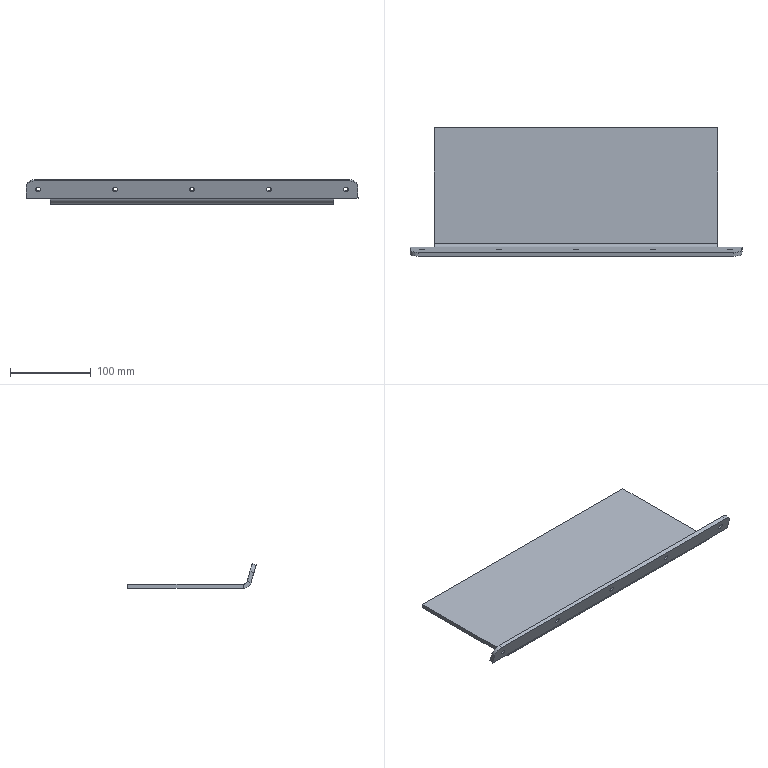Part | SolidWorks | features 3DProfileFeature 1, EdgeFlange 1, Fillet 1, FlatPattern 1, HoleWzd 1, LPattern 1, SMBaseFlange 1, SheetMetal 1 | 1 solid | 38 faces | box 410 x 158.498 x 30.188 mm | volume 311527 mm3 | cylinder 14 | plane 14 | cone 10 | commonest cylinder face diameters 6 x10 20 x3 10 x1
STEP:
#1=CARTESIAN_POINT('',(190.,-81.218,21.139));
#2=VERTEX_POINT('',#1);
#3=CARTESIAN_POINT('',(190.,-79.518,15.385));
#4=VERTEX_POINT('',#3);
#5=CARTESIAN_POINT('',(190.,-80.368,18.262));
#6=DIRECTION('',(0.,-0.959,-0.2833));
#7=DIRECTION('',(0.,0.2833,-0.959));
#8=AXIS2_PLACEMENT_3D('',#5,#6,#7);
#9=CIRCLE('',#8,3.);
#10=EDGE_CURVE('',#2,#4,#9,.T.);
#11=ORIENTED_EDGE('',*,*,#10,.F.);
#12=CARTESIAN_POINT('',(190.,-81.249,21.156));
#13=VERTEX_POINT('',#12);
#14=CARTESIAN_POINT('',(190.,-81.249,21.156));
#15=DIRECTION('',(0.,-0.8784,0.4778));
#16=VECTOR('',#15,1000.);
#17=LINE('',#14,#16);
#18=EDGE_CURVE('',#2,#13,#17,.T.);
#19=ORIENTED_EDGE('',*,*,#18,.T.);
#20=CARTESIAN_POINT('',(190.,-79.535,15.354));
#21=VERTEX_POINT('',#20);
#22=CARTESIAN_POINT('',(190.,-80.392,18.255));
#23=DIRECTION('',(0.,-0.959,-0.2833));
#24=DIRECTION('',(0.,0.2833,-0.959));
#25=AXIS2_PLACEMENT_3D('',#22,#23,#24);
#26=CIRCLE('',#25,3.025);
#27=EDGE_CURVE('',#13,#21,#26,.T.);
#28=ORIENTED_EDGE('',*,*,#27,.T.);
#29=CARTESIAN_POINT('',(190.,-79.535,15.354));
#30=DIRECTION('',(0.,-0.4778,-0.8784));
#31=VECTOR('',#30,1000.);
#32=LINE('',#29,#31);
#33=EDGE_CURVE('',#4,#21,#32,.T.);
#34=ORIENTED_EDGE('',*,*,#33,.F.);
#35=EDGE_LOOP('',(#11,#19,#28,#34));
#36=FACE_OUTER_BOUND('',#35,.T.);
#37=CARTESIAN_POINT('',(190.,-80.392,18.255));
#38=DIRECTION('',(0.,-0.959,-0.2833));
#39=DIRECTION('',(0.,0.2833,-0.959));
#40=AXIS2_PLACEMENT_3D('',#37,#38,#39);
#41=CONICAL_SURFACE('',#40,3.025,0.7854);
#42=ADVANCED_FACE('',(#36),#41,.F.);
#43=CARTESIAN_POINT('',(190.,-76.447,22.549));
#44=VERTEX_POINT('',#43);
#45=CARTESIAN_POINT('',(190.,-74.747,16.794));
#46=VERTEX_POINT('',#45);
#47=CARTESIAN_POINT('',(190.,-75.597,19.671));
#48=DIRECTION('',(0.,-0.959,-0.2833));
#49=DIRECTION('',(0.,0.2833,-0.959));
#50=AXIS2_PLACEMENT_3D('',#47,#48,#49);
#51=CIRCLE('',#50,3.);
#52=EDGE_CURVE('',#44,#46,#51,.T.);
#53=ORIENTED_EDGE('',*,*,#52,.F.);
#54=CARTESIAN_POINT('',(190.,-81.242,21.132));
#55=DIRECTION('',(0.,-0.959,-0.2833));
#56=VECTOR('',#55,1000.);
#57=LINE('',#54,#56);
#58=EDGE_CURVE('',#44,#2,#57,.T.);
#59=ORIENTED_EDGE('',*,*,#58,.T.);
#60=ORIENTED_EDGE('',*,*,#10,.T.);
#61=CARTESIAN_POINT('',(190.,-79.542,15.378));
#62=DIRECTION('',(0.,-0.959,-0.2833));
#63=VECTOR('',#62,1000.);
#64=LINE('',#61,#63);
#65=EDGE_CURVE('',#46,#4,#64,.T.);
#66=ORIENTED_EDGE('',*,*,#65,.F.);
#67=EDGE_LOOP('',(#53,#59,#60,#66));
#68=FACE_OUTER_BOUND('',#67,.T.);
#69=CARTESIAN_POINT('',(190.,-80.392,18.255));
#70=DIRECTION('',(0.,-0.959,-0.2833));
#71=DIRECTION('',(0.,0.2833,-0.959));
#72=AXIS2_PLACEMENT_3D('',#69,#70,#71);
#73=CYLINDRICAL_SURFACE('',#72,3.);
#74=ADVANCED_FACE('',(#68),#73,.F.);
#75=CARTESIAN_POINT('',(95.,-81.218,21.139));
#76=VERTEX_POINT('',#75);
#77=CARTESIAN_POINT('',(95.,-79.518,15.385));
#78=VERTEX_POINT('',#77);
#79=CARTESIAN_POINT('',(95.,-80.368,18.262));
#80=DIRECTION('',(0.,-0.959,-0.2833));
#81=DIRECTION('',(0.,0.2833,-0.959));
#82=AXIS2_PLACEMENT_3D('',#79,#80,#81);
#83=CIRCLE('',#82,3.);
#84=EDGE_CURVE('',#76,#78,#83,.T.);
#85=ORIENTED_EDGE('',*,*,#84,.F.);
#86=CARTESIAN_POINT('',(95.,-81.249,21.156));
#87=VERTEX_POINT('',#86);
#88=CARTESIAN_POINT('',(95.,-81.249,21.156));
#89=DIRECTION('',(0.,-0.8784,0.4778));
#90=VECTOR('',#89,1000.);
#91=LINE('',#88,#90);
#92=EDGE_CURVE('',#76,#87,#91,.T.);
#93=ORIENTED_EDGE('',*,*,#92,.T.);
#94=CARTESIAN_POINT('',(95.,-79.535,15.354));
#95=VERTEX_POINT('',#94);
#96=CARTESIAN_POINT('',(95.,-80.392,18.255));
#97=DIRECTION('',(0.,-0.959,-0.2833));
#98=DIRECTION('',(0.,0.2833,-0.959));
#99=AXIS2_PLACEMENT_3D('',#96,#97,#98);
#100=CIRCLE('',#99,3.025);
#101=EDGE_CURVE('',#87,#95,#100,.T.);
#102=ORIENTED_EDGE('',*,*,#101,.T.);
#103=CARTESIAN_POINT('',(95.,-79.535,15.354));
#104=DIRECTION('',(0.,-0.4778,-0.8784));
#105=VECTOR('',#104,1000.);
#106=LINE('',#103,#105);
#107=EDGE_CURVE('',#78,#95,#106,.T.);
#108=ORIENTED_EDGE('',*,*,#107,.F.);
#109=EDGE_LOOP('',(#85,#93,#102,#108));
#110=FACE_OUTER_BOUND('',#109,.T.);
#111=CARTESIAN_POINT('',(95.,-80.392,18.255));
#112=DIRECTION('',(0.,-0.959,-0.2833));
#113=DIRECTION('',(0.,0.2833,-0.959));
#114=AXIS2_PLACEMENT_3D('',#111,#112,#113);
#115=CONICAL_SURFACE('',#114,3.025,0.7854);
#116=ADVANCED_FACE('',(#110),#115,.F.);
#117=CARTESIAN_POINT('',(95.,-76.447,22.549));
#118=VERTEX_POINT('',#117);
#119=CARTESIAN_POINT('',(95.,-74.747,16.794));
#120=VERTEX_POINT('',#119);
#121=CARTESIAN_POINT('',(95.,-75.597,19.671));
#122=DIRECTION('',(0.,-0.959,-0.2833));
#123=DIRECTION('',(0.,0.2833,-0.959));
#124=AXIS2_PLACEMENT_3D('',#121,#122,#123);
#125=CIRCLE('',#124,3.);
#126=EDGE_CURVE('',#118,#120,#125,.T.);
#127=ORIENTED_EDGE('',*,*,#126,.F.);
#128=CARTESIAN_POINT('',(95.,-81.242,21.132));
#129=DIRECTION('',(0.,-0.959,-0.2833));
#130=VECTOR('',#129,1000.);
#131=LINE('',#128,#130);
#132=EDGE_CURVE('',#118,#76,#131,.T.);
#133=ORIENTED_EDGE('',*,*,#132,.T.);
#134=ORIENTED_EDGE('',*,*,#84,.T.);
#135=CARTESIAN_POINT('',(95.,-79.542,15.378));
#136=DIRECTION('',(0.,-0.959,-0.2833));
#137=VECTOR('',#136,1000.);
#138=LINE('',#135,#137);
#139=EDGE_CURVE('',#120,#78,#138,.T.);
#140=ORIENTED_EDGE('',*,*,#139,.F.);
#141=EDGE_LOOP('',(#127,#133,#134,#140));
#142=FACE_OUTER_BOUND('',#141,.T.);
#143=CARTESIAN_POINT('',(95.,-80.392,18.255));
#144=DIRECTION('',(0.,-0.959,-0.2833));
#145=DIRECTION('',(0.,0.2833,-0.959));
#146=AXIS2_PLACEMENT_3D('',#143,#144,#145);
#147=CYLINDRICAL_SURFACE('',#146,3.);
#148=ADVANCED_FACE('',(#142),#147,.F.);
#149=CARTESIAN_POINT('',(0.,-81.218,21.139));
#150=VERTEX_POINT('',#149);
#151=CARTESIAN_POINT('',(0.,-79.518,15.385));
#152=VERTEX_POINT('',#151);
#153=CARTESIAN_POINT('',(0.,-80.368,18.262));
#154=DIRECTION('',(0.,-0.959,-0.2833));
#155=DIRECTION('',(0.,0.2833,-0.959));
#156=AXIS2_PLACEMENT_3D('',#153,#154,#155);
#157=CIRCLE('',#156,3.);
#158=EDGE_CURVE('',#150,#152,#157,.T.);
#159=ORIENTED_EDGE('',*,*,#158,.F.);
#160=CARTESIAN_POINT('',(0.,-81.249,21.156));
#161=VERTEX_POINT('',#160);
#162=CARTESIAN_POINT('',(0.,-81.249,21.156));
#163=DIRECTION('',(0.,-0.8784,0.4778));
#164=VECTOR('',#163,1000.);
#165=LINE('',#162,#164);
#166=EDGE_CURVE('',#150,#161,#165,.T.);
#167=ORIENTED_EDGE('',*,*,#166,.T.);
#168=CARTESIAN_POINT('',(0.,-79.535,15.354));
#169=VERTEX_POINT('',#168);
#170=CARTESIAN_POINT('',(0.,-80.392,18.255));
#171=DIRECTION('',(0.,-0.959,-0.2833));
#172=DIRECTION('',(0.,0.2833,-0.959));
#173=AXIS2_PLACEMENT_3D('',#170,#171,#172);
#174=CIRCLE('',#173,3.025);
#175=EDGE_CURVE('',#161,#169,#174,.T.);
#176=ORIENTED_EDGE('',*,*,#175,.T.);
#177=CARTESIAN_POINT('',(0.,-79.535,15.354));
#178=DIRECTION('',(0.,-0.4778,-0.8784));
#179=VECTOR('',#178,1000.);
#180=LINE('',#177,#179);
#181=EDGE_CURVE('',#152,#169,#180,.T.);
#182=ORIENTED_EDGE('',*,*,#181,.F.);
#183=EDGE_LOOP('',(#159,#167,#176,#182));
#184=FACE_OUTER_BOUND('',#183,.T.);
#185=CARTESIAN_POINT('',(0.,-80.392,18.255));
#186=DIRECTION('',(0.,-0.959,-0.2833));
#187=DIRECTION('',(0.,0.2833,-0.959));
#188=AXIS2_PLACEMENT_3D('',#185,#186,#187);
#189=CONICAL_SURFACE('',#188,3.025,0.7854);
#190=ADVANCED_FACE('',(#184),#189,.F.);
#191=CARTESIAN_POINT('',(0.,-76.447,22.549));
#192=VERTEX_POINT('',#191);
#193=CARTESIAN_POINT('',(0.,-74.747,16.794));
#194=VERTEX_POINT('',#193);
#195=CARTESIAN_POINT('',(0.,-75.597,19.671));
#196=DIRECTION('',(0.,-0.959,-0.2833));
#197=DIRECTION('',(0.,0.2833,-0.959));
#198=AXIS2_PLACEMENT_3D('',#195,#196,#197);
#199=CIRCLE('',#198,3.);
#200=EDGE_CURVE('',#192,#194,#199,.T.);
#201=ORIENTED_EDGE('',*,*,#200,.F.);
#202=CARTESIAN_POINT('',(0.,-81.242,21.132));
#203=DIRECTION('',(0.,-0.959,-0.2833));
#204=VECTOR('',#203,1000.);
#205=LINE('',#202,#204);
#206=EDGE_CURVE('',#192,#150,#205,.T.);
#207=ORIENTED_EDGE('',*,*,#206,.T.);
#208=ORIENTED_EDGE('',*,*,#158,.T.);
#209=CARTESIAN_POINT('',(0.,-79.542,15.378));
#210=DIRECTION('',(0.,-0.959,-0.2833));
#211=VECTOR('',#210,1000.);
#212=LINE('',#209,#211);
#213=EDGE_CURVE('',#194,#152,#212,.T.);
#214=ORIENTED_EDGE('',*,*,#213,.F.);
#215=EDGE_LOOP('',(#201,#207,#208,#214));
#216=FACE_OUTER_BOUND('',#215,.T.);
#217=CARTESIAN_POINT('',(0.,-80.392,18.255));
#218=DIRECTION('',(0.,-0.959,-0.2833));
#219=DIRECTION('',(0.,0.2833,-0.959));
#220=AXIS2_PLACEMENT_3D('',#217,#218,#219);
#221=CYLINDRICAL_SURFACE('',#220,3.);
#222=ADVANCED_FACE('',(#216),#221,.F.);
#223=CARTESIAN_POINT('',(-95.,-81.218,21.139));
#224=VERTEX_POINT('',#223);
#225=CARTESIAN_POINT('',(-95.,-79.518,15.385));
#226=VERTEX_POINT('',#225);
#227=CARTESIAN_POINT('',(-95.,-80.368,18.262));
#228=DIRECTION('',(0.,-0.959,-0.2833));
#229=DIRECTION('',(0.,0.2833,-0.959));
#230=AXIS2_PLACEMENT_3D('',#227,#228,#229);
#231=CIRCLE('',#230,3.);
#232=EDGE_CURVE('',#224,#226,#231,.T.);
#233=ORIENTED_EDGE('',*,*,#232,.F.);
#234=CARTESIAN_POINT('',(-95.,-81.249,21.156));
#235=VERTEX_POINT('',#234);
#236=CARTESIAN_POINT('',(-95.,-81.249,21.156));
#237=DIRECTION('',(0.,-0.8784,0.4778));
#238=VECTOR('',#237,1000.);
#239=LINE('',#236,#238);
#240=EDGE_CURVE('',#224,#235,#239,.T.);
#241=ORIENTED_EDGE('',*,*,#240,.T.);
#242=CARTESIAN_POINT('',(-95.,-79.535,15.354));
#243=VERTEX_POINT('',#242);
#244=CARTESIAN_POINT('',(-95.,-80.392,18.255));
#245=DIRECTION('',(0.,-0.959,-0.2833));
#246=DIRECTION('',(0.,0.2833,-0.959));
#247=AXIS2_PLACEMENT_3D('',#244,#245,#246);
#248=CIRCLE('',#247,3.025);
#249=EDGE_CURVE('',#235,#243,#248,.T.);
#250=ORIENTED_EDGE('',*,*,#249,.T.);
#251=CARTESIAN_POINT('',(-95.,-79.535,15.354));
#252=DIRECTION('',(0.,-0.4778,-0.8784));
#253=VECTOR('',#252,1000.);
#254=LINE('',#251,#253);
#255=EDGE_CURVE('',#226,#243,#254,.T.);
#256=ORIENTED_EDGE('',*,*,#255,.F.);
#257=EDGE_LOOP('',(#233,#241,#250,#256));
#258=FACE_OUTER_BOUND('',#257,.T.);
#259=CARTESIAN_POINT('',(-95.,-80.392,18.255));
#260=DIRECTION('',(0.,-0.959,-0.2833));
#261=DIRECTION('',(0.,0.2833,-0.959));
#262=AXIS2_PLACEMENT_3D('',#259,#260,#261);
#263=CONICAL_SURFACE('',#262,3.025,0.7854);
#264=ADVANCED_FACE('',(#258),#263,.F.);
#265=CARTESIAN_POINT('',(-95.,-76.447,22.549));
#266=VERTEX_POINT('',#265);
#267=CARTESIAN_POINT('',(-95.,-74.747,16.794));
#268=VERTEX_POINT('',#267);
#269=CARTESIAN_POINT('',(-95.,-75.597,19.671));
#270=DIRECTION('',(0.,-0.959,-0.2833));
#271=DIRECTION('',(0.,0.2833,-0.959));
#272=AXIS2_PLACEMENT_3D('',#269,#270,#271);
#273=CIRCLE('',#272,3.);
#274=EDGE_CURVE('',#266,#268,#273,.T.);
#275=ORIENTED_EDGE('',*,*,#274,.F.);
#276=CARTESIAN_POINT('',(-95.,-81.242,21.132));
#277=DIRECTION('',(0.,-0.959,-0.2833));
#278=VECTOR('',#277,1000.);
#279=LINE('',#276,#278);
#280=EDGE_CURVE('',#266,#224,#279,.T.);
#281=ORIENTED_EDGE('',*,*,#280,.T.);
#282=ORIENTED_EDGE('',*,*,#232,.T.);
#283=CARTESIAN_POINT('',(-95.,-79.542,15.378));
#284=DIRECTION('',(0.,-0.959,-0.2833));
#285=VECTOR('',#284,1000.);
#286=LINE('',#283,#285);
#287=EDGE_CURVE('',#268,#226,#286,.T.);
#288=ORIENTED_EDGE('',*,*,#287,.F.);
#289=EDGE_LOOP('',(#275,#281,#282,#288));
#290=FACE_OUTER_BOUND('',#289,.T.);
#291=CARTESIAN_POINT('',(-95.,-80.392,18.255));
#292=DIRECTION('',(0.,-0.959,-0.2833));
#293=DIRECTION('',(0.,0.2833,-0.959));
#294=AXIS2_PLACEMENT_3D('',#291,#292,#293);
#295=CYLINDRICAL_SURFACE('',#294,3.);
#296=ADVANCED_FACE('',(#290),#295,.F.);
#297=CARTESIAN_POINT('',(-190.,-81.218,21.139));
#298=VERTEX_POINT('',#297);
#299=CARTESIAN_POINT('',(-190.,-79.518,15.385));
#300=VERTEX_POINT('',#299);
#301=CARTESIAN_POINT('',(-190.,-80.368,18.262));
#302=DIRECTION('',(0.,-0.959,-0.2833));
#303=DIRECTION('',(0.,0.2833,-0.959));
#304=AXIS2_PLACEMENT_3D('',#301,#302,#303);
#305=CIRCLE('',#304,3.);
#306=EDGE_CURVE('',#298,#300,#305,.T.);
#307=ORIENTED_EDGE('',*,*,#306,.F.);
#308=CARTESIAN_POINT('',(-190.,-81.249,21.156));
#309=VERTEX_POINT('',#308);
#310=CARTESIAN_POINT('',(-190.,-81.249,21.156));
#311=DIRECTION('',(0.,-0.8784,0.4778));
#312=VECTOR('',#311,1000.);
#313=LINE('',#310,#312);
#314=EDGE_CURVE('',#298,#309,#313,.T.);
#315=ORIENTED_EDGE('',*,*,#314,.T.);
#316=CARTESIAN_POINT('',(-190.,-79.535,15.354));
#317=VERTEX_POINT('',#316);
#318=CARTESIAN_POINT('',(-190.,-80.392,18.255));
#319=DIRECTION('',(0.,-0.959,-0.2833));
#320=DIRECTION('',(0.,0.2833,-0.959));
#321=AXIS2_PLACEMENT_3D('',#318,#319,#320);
#322=CIRCLE('',#321,3.025);
#323=EDGE_CURVE('',#309,#317,#322,.T.);
#324=ORIENTED_EDGE('',*,*,#323,.T.);
#325=CARTESIAN_POINT('',(-190.,-79.535,15.354));
#326=DIRECTION('',(0.,-0.4778,-0.8784));
#327=VECTOR('',#326,1000.);
#328=LINE('',#325,#327);
#329=EDGE_CURVE('',#300,#317,#328,.T.);
#330=ORIENTED_EDGE('',*,*,#329,.F.);
#331=EDGE_LOOP('',(#307,#315,#324,#330));
#332=FACE_OUTER_BOUND('',#331,.T.);
#333=CARTESIAN_POINT('',(-190.,-80.392,18.255));
#334=DIRECTION('',(0.,-0.959,-0.2833));
#335=DIRECTION('',(0.,0.2833,-0.959));
#336=AXIS2_PLACEMENT_3D('',#333,#334,#335);
#337=CONICAL_SURFACE('',#336,3.025,0.7854);
#338=ADVANCED_FACE('',(#332),#337,.F.);
#339=CARTESIAN_POINT('',(-190.,-76.447,22.549));
#340=VERTEX_POINT('',#339);
#341=CARTESIAN_POINT('',(-190.,-74.747,16.794));
#342=VERTEX_POINT('',#341);
#343=CARTESIAN_POINT('',(-190.,-75.597,19.671));
#344=DIRECTION('',(0.,-0.959,-0.2833));
#345=DIRECTION('',(0.,0.2833,-0.959));
#346=AXIS2_PLACEMENT_3D('',#343,#344,#345);
#347=CIRCLE('',#346,3.);
#348=EDGE_CURVE('',#340,#342,#347,.T.);
#349=ORIENTED_EDGE('',*,*,#348,.F.);
#350=CARTESIAN_POINT('',(-190.,-81.242,21.132));
#351=DIRECTION('',(0.,-0.959,-0.2833));
#352=VECTOR('',#351,1000.);
#353=LINE('',#350,#352);
#354=EDGE_CURVE('',#340,#298,#353,.T.);
#355=ORIENTED_EDGE('',*,*,#354,.T.);
#356=ORIENTED_EDGE('',*,*,#306,.T.);
#357=CARTESIAN_POINT('',(-190.,-79.542,15.378));
#358=DIRECTION('',(0.,-0.959,-0.2833));
#359=VECTOR('',#358,1000.);
#360=LINE('',#357,#359);
#361=EDGE_CURVE('',#342,#300,#360,.T.);
#362=ORIENTED_EDGE('',*,*,#361,.F.);
#363=EDGE_LOOP('',(#349,#355,#356,#362));
#364=FACE_OUTER_BOUND('',#363,.T.);
#365=CARTESIAN_POINT('',(-190.,-80.392,18.255));
#366=DIRECTION('',(0.,-0.959,-0.2833));
#367=DIRECTION('',(0.,0.2833,-0.959));
#368=AXIS2_PLACEMENT_3D('',#365,#366,#367);
#369=CYLINDRICAL_SURFACE('',#368,3.);
#370=ADVANCED_FACE('',(#364),#369,.F.);
#371=CARTESIAN_POINT('',(175.,-67.527,5.));
#372=VERTEX_POINT('',#371);
#373=CARTESIAN_POINT('',(175.,-67.527,0.));
#374=VERTEX_POINT('',#373);
#375=CARTESIAN_POINT('',(175.,-67.527,5.));
#376=DIRECTION('',(0.,0.,-1.));
#377=VECTOR('',#376,1000.);
#378=LINE('',#375,#377);
#379=EDGE_CURVE('',#372,#374,#378,.T.);
#380=ORIENTED_EDGE('',*,*,#379,.T.);
#381=CARTESIAN_POINT('',(175.,75.,0.));
#382=VERTEX_POINT('',#381);
#383=CARTESIAN_POINT('',(175.,75.,0.));
#384=DIRECTION('',(0.,1.,0.));
#385=VECTOR('',#384,1000.);
#386=LINE('',#383,#385);
#387=EDGE_CURVE('',#374,#382,#386,.T.);
#388=ORIENTED_EDGE('',*,*,#387,.T.);
#389=CARTESIAN_POINT('',(175.,75.,5.));
#390=VERTEX_POINT('',#389);
#391=CARTESIAN_POINT('',(175.,75.,5.));
#392=DIRECTION('',(0.,0.,-1.));
#393=VECTOR('',#392,1000.);
#394=LINE('',#391,#393);
#395=EDGE_CURVE('',#390,#382,#394,.T.);
#396=ORIENTED_EDGE('',*,*,#395,.F.);
#397=CARTESIAN_POINT('',(175.,75.,5.));
#398=DIRECTION('',(0.,1.,0.));
#399=VECTOR('',#398,1000.);
#400=LINE('',#397,#399);
#401=EDGE_CURVE('',#372,#390,#400,.T.);
#402=ORIENTED_EDGE('',*,*,#401,.F.);
#403=EDGE_LOOP('',(#380,#388,#396,#402));
#404=FACE_OUTER_BOUND('',#403,.T.);
#405=CARTESIAN_POINT('',(175.,75.,5.));
#406=DIRECTION('',(-1.,0.,0.));
#407=DIRECTION('',(0.,0.,1.));
#408=AXIS2_PLACEMENT_3D('',#405,#406,#407);
#409=PLANE('',#408);
#410=ADVANCED_FACE('',(#404),#409,.F.);
#411=CARTESIAN_POINT('',(-175.,-67.527,5.));
#412=VERTEX_POINT('',#411);
#413=CARTESIAN_POINT('',(-175.,-67.527,0.));
#414=VERTEX_POINT('',#413);
#415=CARTESIAN_POINT('',(-175.,-67.527,5.));
#416=DIRECTION('',(0.,0.,-1.));
#417=VECTOR('',#416,1000.);
#418=LINE('',#415,#417);
#419=EDGE_CURVE('',#412,#414,#418,.T.);
#420=ORIENTED_EDGE('',*,*,#419,.F.);
#421=CARTESIAN_POINT('',(-175.,75.,5.));
#422=VERTEX_POINT('',#421);
#423=CARTESIAN_POINT('',(-175.,75.,5.));
#424=DIRECTION('',(0.,-1.,0.));
#425=VECTOR('',#424,1000.);
#426=LINE('',#423,#425);
#427=EDGE_CURVE('',#422,#412,#426,.T.);
#428=ORIENTED_EDGE('',*,*,#427,.F.);
#429=CARTESIAN_POINT('',(-175.,75.,0.));
#430=VERTEX_POINT('',#429);
#431=CARTESIAN_POINT('',(-175.,75.,5.));
#432=DIRECTION('',(0.,0.,-1.));
#433=VECTOR('',#432,1000.);
#434=LINE('',#431,#433);
#435=EDGE_CURVE('',#422,#430,#434,.T.);
#436=ORIENTED_EDGE('',*,*,#435,.T.);
#437=CARTESIAN_POINT('',(-175.,75.,0.));
#438=DIRECTION('',(0.,-1.,0.));
#439=VECTOR('',#438,1000.);
#440=LINE('',#437,#439);
#441=EDGE_CURVE('',#430,#414,#440,.T.);
#442=ORIENTED_EDGE('',*,*,#441,.T.);
#443=EDGE_LOOP('',(#420,#428,#436,#442));
#444=FACE_OUTER_BOUND('',#443,.T.);
#445=CARTESIAN_POINT('',(-175.,75.,5.));
#446=DIRECTION('',(1.,0.,0.));
#447=DIRECTION('',(0.,0.,-1.));
#448=AXIS2_PLACEMENT_3D('',#445,#446,#447);
#449=PLANE('',#448);
#450=ADVANCED_FACE('',(#444),#449,.F.);
#451=ORIENTED_EDGE('',*,*,#427,.T.);
#452=CARTESIAN_POINT('',(175.,-67.527,5.));
#453=DIRECTION('',(-1.,0.,0.));
#454=VECTOR('',#453,1000.);
#455=LINE('',#452,#454);
#456=EDGE_CURVE('',#372,#412,#455,.T.);
#457=ORIENTED_EDGE('',*,*,#456,.F.);
#458=ORIENTED_EDGE('',*,*,#401,.T.);
#459=CARTESIAN_POINT('',(-175.,75.,5.));
#460=DIRECTION('',(-1.,0.,0.));
#461=VECTOR('',#460,1000.);
#462=LINE('',#459,#461);
#463=EDGE_CURVE('',#390,#422,#462,.T.);
#464=ORIENTED_EDGE('',*,*,#463,.T.);
#465=EDGE_LOOP('',(#451,#457,#458,#464));
#466=FACE_OUTER_BOUND('',#465,.T.);
#467=CARTESIAN_POINT('',(0.,0.,5.));
#468=DIRECTION('',(0.,0.,1.));
#469=DIRECTION('',(1.,0.,0.));
#470=AXIS2_PLACEMENT_3D('',#467,#468,#469);
#471=PLANE('',#470);
#472=ADVANCED_FACE('',(#466),#471,.T.);
#473=CARTESIAN_POINT('',(175.,-67.527,0.));
#474=DIRECTION('',(-1.,0.,0.));
#475=VECTOR('',#474,1000.);
#476=LINE('',#473,#475);
#477=EDGE_CURVE('',#374,#414,#476,.T.);
#478=ORIENTED_EDGE('',*,*,#477,.T.);
#479=ORIENTED_EDGE('',*,*,#441,.F.);
#480=CARTESIAN_POINT('',(-175.,75.,0.));
#481=DIRECTION('',(-1.,0.,0.));
#482=VECTOR('',#481,1000.);
#483=LINE('',#480,#482);
#484=EDGE_CURVE('',#382,#430,#483,.T.);
#485=ORIENTED_EDGE('',*,*,#484,.F.);
#486=ORIENTED_EDGE('',*,*,#387,.F.);
#487=EDGE_LOOP('',(#478,#479,#485,#486));
#488=FACE_OUTER_BOUND('',#487,.T.);
#489=CARTESIAN_POINT('',(0.,0.,0.));
#490=DIRECTION('',(0.,0.,1.));
#491=DIRECTION('',(1.,0.,0.));
#492=AXIS2_PLACEMENT_3D('',#489,#490,#491);
#493=PLANE('',#492);
#494=ADVANCED_FACE('',(#488),#493,.F.);
#495=ORIENTED_EDGE('',*,*,#484,.T.);
#496=ORIENTED_EDGE('',*,*,#435,.F.);
#497=ORIENTED_EDGE('',*,*,#463,.F.);
#498=ORIENTED_EDGE('',*,*,#395,.T.);
#499=EDGE_LOOP('',(#495,#496,#497,#498));
#500=FACE_OUTER_BOUND('',#499,.T.);
#501=CARTESIAN_POINT('',(-175.,75.,5.));
#502=DIRECTION('',(0.,-1.,0.));
#503=DIRECTION('',(0.,0.,-1.));
#504=AXIS2_PLACEMENT_3D('',#501,#502,#503);
#505=PLANE('',#504);
#506=ADVANCED_FACE('',(#500),#505,.F.);
#507=CARTESIAN_POINT('',(-175.,-72.322,8.584));
#508=VERTEX_POINT('',#507);
#509=CARTESIAN_POINT('',(-175.,-77.117,7.167));
#510=VERTEX_POINT('',#509);
#511=CARTESIAN_POINT('',(-175.,-72.322,8.584));
#512=DIRECTION('',(0.,-0.959,-0.2833));
#513=VECTOR('',#512,1000.);
#514=LINE('',#511,#513);
#515=EDGE_CURVE('',#508,#510,#514,.T.);
#516=ORIENTED_EDGE('',*,*,#515,.F.);
#517=CARTESIAN_POINT('',(-175.,-67.527,10.));
#518=DIRECTION('',(-1.,0.,0.));
#519=DIRECTION('',(0.,0.,-1.));
#520=AXIS2_PLACEMENT_3D('',#517,#518,#519);
#521=CIRCLE('',#520,5.);
#522=EDGE_CURVE('',#412,#508,#521,.T.);
#523=ORIENTED_EDGE('',*,*,#522,.F.);
#524=ORIENTED_EDGE('',*,*,#419,.T.);
#525=CARTESIAN_POINT('',(-175.,-67.527,10.));
#526=DIRECTION('',(-1.,0.,0.));
#527=DIRECTION('',(0.,0.,-1.));
#528=AXIS2_PLACEMENT_3D('',#525,#526,#527);
#529=CIRCLE('',#528,10.);
#530=EDGE_CURVE('',#414,#510,#529,.T.);
#531=ORIENTED_EDGE('',*,*,#530,.T.);
#532=EDGE_LOOP('',(#516,#523,#524,#531));
#533=FACE_OUTER_BOUND('',#532,.T.);
#534=CARTESIAN_POINT('',(-175.,-67.527,10.));
#535=DIRECTION('',(-1.,0.,0.));
#536=DIRECTION('',(0.,0.,1.));
#537=AXIS2_PLACEMENT_3D('',#534,#535,#536);
#538=PLANE('',#537);
#539=ADVANCED_FACE('',(#533),#538,.T.);
#540=CARTESIAN_POINT('',(175.,-72.322,8.584));
#541=VERTEX_POINT('',#540);
#542=CARTESIAN_POINT('',(175.,-67.527,10.));
#543=DIRECTION('',(1.,0.,0.));
#544=DIRECTION('',(0.,0.,-1.));
#545=AXIS2_PLACEMENT_3D('',#542,#543,#544);
#546=CIRCLE('',#545,5.);
#547=EDGE_CURVE('',#541,#372,#546,.T.);
#548=ORIENTED_EDGE('',*,*,#547,.F.);
#549=CARTESIAN_POINT('',(175.,-77.117,7.167));
#550=VERTEX_POINT('',#549);
#551=CARTESIAN_POINT('',(175.,-72.322,8.584));
#552=DIRECTION('',(0.,-0.959,-0.2833));
#553=VECTOR('',#552,1000.);
#554=LINE('',#551,#553);
#555=EDGE_CURVE('',#541,#550,#554,.T.);
#556=ORIENTED_EDGE('',*,*,#555,.T.);
#557=CARTESIAN_POINT('',(175.,-67.527,10.));
#558=DIRECTION('',(1.,0.,0.));
#559=DIRECTION('',(0.,0.,-1.));
#560=AXIS2_PLACEMENT_3D('',#557,#558,#559);
#561=CIRCLE('',#560,10.);
#562=EDGE_CURVE('',#550,#374,#561,.T.);
#563=ORIENTED_EDGE('',*,*,#562,.T.);
#564=ORIENTED_EDGE('',*,*,#379,.F.);
#565=EDGE_LOOP('',(#548,#556,#563,#564));
#566=FACE_OUTER_BOUND('',#565,.T.);
#567=CARTESIAN_POINT('',(175.,-67.527,10.));
#568=DIRECTION('',(-1.,0.,0.));
#569=DIRECTION('',(0.,0.,1.));
#570=AXIS2_PLACEMENT_3D('',#567,#568,#569);
#571=PLANE('',#570);
#572=ADVANCED_FACE('',(#566),#571,.F.);
#573=ORIENTED_EDGE('',*,*,#477,.F.);
#574=ORIENTED_EDGE('',*,*,#562,.F.);
#575=CARTESIAN_POINT('',(175.,-77.117,7.167));
#576=DIRECTION('',(1.,0.,0.));
#577=VECTOR('',#576,1000.);
#578=LINE('',#575,#577);
#579=EDGE_CURVE('',#510,#550,#578,.T.);
#580=ORIENTED_EDGE('',*,*,#579,.F.);
#581=ORIENTED_EDGE('',*,*,#530,.F.);
#582=EDGE_LOOP('',(#573,#574,#580,#581));
#583=FACE_OUTER_BOUND('',#582,.T.);
#584=CARTESIAN_POINT('',(175.,-67.527,10.));
#585=DIRECTION('',(1.,0.,0.));
#586=DIRECTION('',(0.,-0.959,-0.2833));
#587=AXIS2_PLACEMENT_3D('',#584,#585,#586);
#588=CYLINDRICAL_SURFACE('',#587,10.);
#589=ADVANCED_FACE('',(#583),#588,.T.);
#590=ORIENTED_EDGE('',*,*,#456,.T.);
#591=ORIENTED_EDGE('',*,*,#522,.T.);
#592=CARTESIAN_POINT('',(175.,-72.322,8.584));
#593=DIRECTION('',(1.,0.,0.));
#594=VECTOR('',#593,1000.);
#595=LINE('',#592,#594);
#596=EDGE_CURVE('',#508,#541,#595,.T.);
#597=ORIENTED_EDGE('',*,*,#596,.T.);
#598=ORIENTED_EDGE('',*,*,#547,.T.);
#599=EDGE_LOOP('',(#590,#591,#597,#598));
#600=FACE_OUTER_BOUND('',#599,.T.);
#601=CARTESIAN_POINT('',(175.,-67.527,10.));
#602=DIRECTION('',(1.,0.,0.));
#603=DIRECTION('',(0.,-0.959,-0.2833));
#604=AXIS2_PLACEMENT_3D('',#601,#602,#603);
#605=CYLINDRICAL_SURFACE('',#604,5.);
#606=ADVANCED_FACE('',(#600),#605,.F.);
#607=ORIENTED_EDGE('',*,*,#555,.F.);
#608=CARTESIAN_POINT('',(205.,-72.322,8.584));
#609=VERTEX_POINT('',#608);
#610=CARTESIAN_POINT('',(-205.,-72.322,8.584));
#611=DIRECTION('',(1.,0.,0.));
#612=VECTOR('',#611,1000.);
#613=LINE('',#610,#612);
#614=EDGE_CURVE('',#541,#609,#613,.T.);
#615=ORIENTED_EDGE('',*,*,#614,.T.);
#616=CARTESIAN_POINT('',(205.,-77.117,7.167));
#617=VERTEX_POINT('',#616);
#618=CARTESIAN_POINT('',(205.,-72.322,8.584));
#619=DIRECTION('',(0.,-0.959,-0.2833));
#620=VECTOR('',#619,1000.);
#621=LINE('',#618,#620);
#622=EDGE_CURVE('',#609,#617,#621,.T.);
#623=ORIENTED_EDGE('',*,*,#622,.T.);
#624=CARTESIAN_POINT('',(0.,-77.117,7.167));
#625=DIRECTION('',(1.,0.,0.));
#626=VECTOR('',#625,1000.);
#627=LINE('',#624,#626);
#628=EDGE_CURVE('',#550,#617,#627,.T.);
#629=ORIENTED_EDGE('',*,*,#628,.F.);
#630=EDGE_LOOP('',(#607,#615,#623,#629));
#631=FACE_OUTER_BOUND('',#630,.T.);
#632=CARTESIAN_POINT('',(-205.,-72.322,8.584));
#633=DIRECTION('',(0.,0.2833,-0.959));
#634=DIRECTION('',(0.,0.959,0.2833));
#635=AXIS2_PLACEMENT_3D('',#632,#633,#634);
#636=PLANE('',#635);
#637=ADVANCED_FACE('',(#631),#636,.T.);
#638=CARTESIAN_POINT('',(205.,-75.87,20.597));
#639=VERTEX_POINT('',#638);
#640=CARTESIAN_POINT('',(205.,-63.887,-19.974));
#641=DIRECTION('',(0.,0.2833,-0.959));
#642=VECTOR('',#641,1000.);
#643=LINE('',#640,#642);
#644=EDGE_CURVE('',#639,#609,#643,.T.);
#645=ORIENTED_EDGE('',*,*,#644,.F.);
#646=CARTESIAN_POINT('',(205.,-80.665,19.181));
#647=VERTEX_POINT('',#646);
#648=CARTESIAN_POINT('',(205.,-80.665,19.181));
#649=DIRECTION('',(0.,-0.959,-0.2833));
#650=VECTOR('',#649,1000.);
#651=LINE('',#648,#650);
#652=EDGE_CURVE('',#639,#647,#651,.T.);
#653=ORIENTED_EDGE('',*,*,#652,.T.);
#654=CARTESIAN_POINT('',(205.,-76.059,3.584));
#655=DIRECTION('',(0.,0.2833,-0.959));
#656=VECTOR('',#655,1000.);
#657=LINE('',#654,#656);
#658=EDGE_CURVE('',#647,#617,#657,.T.);
#659=ORIENTED_EDGE('',*,*,#658,.T.);
#660=ORIENTED_EDGE('',*,*,#622,.F.);
#661=EDGE_LOOP('',(#645,#653,#659,#660));
#662=FACE_OUTER_BOUND('',#661,.T.);
#663=CARTESIAN_POINT('',(205.,-76.059,3.584));
#664=DIRECTION('',(1.,0.,0.));
#665=DIRECTION('',(0.,0.,-1.));
#666=AXIS2_PLACEMENT_3D('',#663,#664,#665);
#667=PLANE('',#666);
#668=ADVANCED_FACE('',(#662),#667,.T.);
#669=CARTESIAN_POINT('',(-205.,-77.117,7.167));
#670=VERTEX_POINT('',#669);
#671=CARTESIAN_POINT('',(-205.,-80.665,19.181));
#672=VERTEX_POINT('',#671);
#673=CARTESIAN_POINT('',(-205.,-83.498,28.771));
#674=DIRECTION('',(0.,-0.2833,0.959));
#675=VECTOR('',#674,1000.);
#676=LINE('',#673,#675);
#677=EDGE_CURVE('',#670,#672,#676,.T.);
#678=ORIENTED_EDGE('',*,*,#677,.T.);
#679=CARTESIAN_POINT('',(-205.,-75.87,20.597));
#680=VERTEX_POINT('',#679);
#681=CARTESIAN_POINT('',(-205.,-80.665,19.181));
#682=DIRECTION('',(0.,0.959,0.2833));
#683=VECTOR('',#682,1000.);
#684=LINE('',#681,#683);
#685=EDGE_CURVE('',#672,#680,#684,.T.);
#686=ORIENTED_EDGE('',*,*,#685,.T.);
#687=CARTESIAN_POINT('',(-205.,-72.322,8.584));
#688=VERTEX_POINT('',#687);
#689=CARTESIAN_POINT('',(-205.,-63.887,-19.974));
#690=DIRECTION('',(0.,-0.2833,0.959));
#691=VECTOR('',#690,1000.);
#692=LINE('',#689,#691);
#693=EDGE_CURVE('',#688,#680,#692,.T.);
#694=ORIENTED_EDGE('',*,*,#693,.F.);
#695=CARTESIAN_POINT('',(-205.,-77.117,7.167));
#696=DIRECTION('',(0.,-0.959,-0.2833));
#697=VECTOR('',#696,1000.);
#698=LINE('',#695,#697);
#699=EDGE_CURVE('',#688,#670,#698,.T.);
#700=ORIENTED_EDGE('',*,*,#699,.T.);
#701=EDGE_LOOP('',(#678,#686,#694,#700));
#702=FACE_OUTER_BOUND('',#701,.T.);
#703=CARTESIAN_POINT('',(-205.,-83.498,28.771));
#704=DIRECTION('',(-1.,0.,0.));
#705=DIRECTION('',(0.,0.,1.));
#706=AXIS2_PLACEMENT_3D('',#703,#704,#705);
#707=PLANE('',#706);
#708=ADVANCED_FACE('',(#702),#707,.T.);
#709=CARTESIAN_POINT('',(190.,-80.392,18.255));
#710=DIRECTION('',(0.,-0.959,-0.2833));
#711=DIRECTION('',(0.,0.2833,-0.959));
#712=AXIS2_PLACEMENT_3D('',#709,#710,#711);
#713=CIRCLE('',#712,3.025);
#714=EDGE_CURVE('',#21,#13,#713,.T.);
#715=ORIENTED_EDGE('',*,*,#714,.F.);
#716=ORIENTED_EDGE('',*,*,#27,.F.);
#717=EDGE_LOOP('',(#715,#716));
#718=FACE_BOUND('',#717,.T.);
#719=CARTESIAN_POINT('',(95.,-80.392,18.255));
#720=DIRECTION('',(0.,-0.959,-0.2833));
#721=DIRECTION('',(0.,0.2833,-0.959));
#722=AXIS2_PLACEMENT_3D('',#719,#720,#721);
#723=CIRCLE('',#722,3.025);
#724=EDGE_CURVE('',#95,#87,#723,.T.);
#725=ORIENTED_EDGE('',*,*,#724,.F.);
#726=ORIENTED_EDGE('',*,*,#101,.F.);
#727=EDGE_LOOP('',(#725,#726));
#728=FACE_BOUND('',#727,.T.);
#729=CARTESIAN_POINT('',(0.,-80.392,18.255));
#730=DIRECTION('',(0.,-0.959,-0.2833));
#731=DIRECTION('',(0.,0.2833,-0.959));
#732=AXIS2_PLACEMENT_3D('',#729,#730,#731);
#733=CIRCLE('',#732,3.025);
#734=EDGE_CURVE('',#169,#161,#733,.T.);
#735=ORIENTED_EDGE('',*,*,#734,.F.);
#736=ORIENTED_EDGE('',*,*,#175,.F.);
#737=EDGE_LOOP('',(#735,#736));
#738=FACE_BOUND('',#737,.T.);
#739=CARTESIAN_POINT('',(-95.,-80.392,18.255));
#740=DIRECTION('',(0.,-0.959,-0.2833));
#741=DIRECTION('',(0.,0.2833,-0.959));
#742=AXIS2_PLACEMENT_3D('',#739,#740,#741);
#743=CIRCLE('',#742,3.025);
#744=EDGE_CURVE('',#243,#235,#743,.T.);
#745=ORIENTED_EDGE('',*,*,#744,.F.);
#746=ORIENTED_EDGE('',*,*,#249,.F.);
#747=EDGE_LOOP('',(#745,#746));
#748=FACE_BOUND('',#747,.T.);
#749=CARTESIAN_POINT('',(-190.,-80.392,18.255));
#750=DIRECTION('',(0.,-0.959,-0.2833));
#751=DIRECTION('',(0.,0.2833,-0.959));
#752=AXIS2_PLACEMENT_3D('',#749,#750,#751);
#753=CIRCLE('',#752,3.025);
#754=EDGE_CURVE('',#317,#309,#753,.T.);
#755=ORIENTED_EDGE('',*,*,#754,.F.);
#756=ORIENTED_EDGE('',*,*,#323,.F.);
#757=EDGE_LOOP('',(#755,#756));
#758=FACE_BOUND('',#757,.T.);
#759=ORIENTED_EDGE('',*,*,#658,.F.);
#760=CARTESIAN_POINT('',(195.,-83.498,28.771));
#761=VERTEX_POINT('',#760);
#762=CARTESIAN_POINT('',(195.,-80.665,19.181));
#763=DIRECTION('',(0.,-0.959,-0.2833));
#764=DIRECTION('',(0.,0.2833,-0.959));
#765=AXIS2_PLACEMENT_3D('',#762,#763,#764);
#766=CIRCLE('',#765,10.);
#767=EDGE_CURVE('',#647,#761,#766,.T.);
#768=ORIENTED_EDGE('',*,*,#767,.T.);
#769=CARTESIAN_POINT('',(-195.,-83.498,28.771));
#770=VERTEX_POINT('',#769);
#771=CARTESIAN_POINT('',(205.,-83.498,28.771));
#772=DIRECTION('',(1.,0.,0.));
#773=VECTOR('',#772,1000.);
#774=LINE('',#771,#773);
#775=EDGE_CURVE('',#770,#761,#774,.T.);
#776=ORIENTED_EDGE('',*,*,#775,.F.);
#777=CARTESIAN_POINT('',(-195.,-80.665,19.181));
#778=DIRECTION('',(0.,-0.959,-0.2833));
#779=DIRECTION('',(0.,0.2833,-0.959));
#780=AXIS2_PLACEMENT_3D('',#777,#778,#779);
#781=CIRCLE('',#780,10.);
#782=EDGE_CURVE('',#770,#672,#781,.T.);
#783=ORIENTED_EDGE('',*,*,#782,.T.);
#784=ORIENTED_EDGE('',*,*,#677,.F.);
#785=CARTESIAN_POINT('',(0.,-77.117,7.167));
#786=DIRECTION('',(1.,0.,0.));
#787=VECTOR('',#786,1000.);
#788=LINE('',#785,#787);
#789=EDGE_CURVE('',#670,#510,#788,.T.);
#790=ORIENTED_EDGE('',*,*,#789,.T.);
#791=ORIENTED_EDGE('',*,*,#579,.T.);
#792=ORIENTED_EDGE('',*,*,#628,.T.);
#793=EDGE_LOOP('',(#759,#768,#776,#783,#784,#790,#791,#792));
#794=FACE_OUTER_BOUND('',#793,.T.);
#795=CARTESIAN_POINT('',(0.,-68.682,-21.39));
#796=DIRECTION('',(0.,-0.959,-0.2833));
#797=DIRECTION('',(0.,0.2833,-0.959));
#798=AXIS2_PLACEMENT_3D('',#795,#796,#797);
#799=PLANE('',#798);
#800=ADVANCED_FACE('',(#718,#728,#738,#748,#758,#794),#799,.T.);
#801=CARTESIAN_POINT('',(190.,-75.597,19.671));
#802=DIRECTION('',(0.,-0.959,-0.2833));
#803=DIRECTION('',(0.,0.2833,-0.959));
#804=AXIS2_PLACEMENT_3D('',#801,#802,#803);
#805=CIRCLE('',#804,3.);
#806=EDGE_CURVE('',#46,#44,#805,.T.);
#807=ORIENTED_EDGE('',*,*,#806,.T.);
#808=ORIENTED_EDGE('',*,*,#52,.T.);
#809=EDGE_LOOP('',(#807,#808));
#810=FACE_BOUND('',#809,.T.);
#811=CARTESIAN_POINT('',(95.,-75.597,19.671));
#812=DIRECTION('',(0.,-0.959,-0.2833));
#813=DIRECTION('',(0.,0.2833,-0.959));
#814=AXIS2_PLACEMENT_3D('',#811,#812,#813);
#815=CIRCLE('',#814,3.);
#816=EDGE_CURVE('',#120,#118,#815,.T.);
#817=ORIENTED_EDGE('',*,*,#816,.T.);
#818=ORIENTED_EDGE('',*,*,#126,.T.);
#819=EDGE_LOOP('',(#817,#818));
#820=FACE_BOUND('',#819,.T.);
#821=CARTESIAN_POINT('',(0.,-75.597,19.671));
#822=DIRECTION('',(0.,-0.959,-0.2833));
#823=DIRECTION('',(0.,0.2833,-0.959));
#824=AXIS2_PLACEMENT_3D('',#821,#822,#823);
#825=CIRCLE('',#824,3.);
#826=EDGE_CURVE('',#194,#192,#825,.T.);
#827=ORIENTED_EDGE('',*,*,#826,.T.);
#828=ORIENTED_EDGE('',*,*,#200,.T.);
#829=EDGE_LOOP('',(#827,#828));
#830=FACE_BOUND('',#829,.T.);
#831=CARTESIAN_POINT('',(-95.,-75.597,19.671));
#832=DIRECTION('',(0.,-0.959,-0.2833));
#833=DIRECTION('',(0.,0.2833,-0.959));
#834=AXIS2_PLACEMENT_3D('',#831,#832,#833);
#835=CIRCLE('',#834,3.);
#836=EDGE_CURVE('',#268,#266,#835,.T.);
#837=ORIENTED_EDGE('',*,*,#836,.T.);
#838=ORIENTED_EDGE('',*,*,#274,.T.);
#839=EDGE_LOOP('',(#837,#838));
#840=FACE_BOUND('',#839,.T.);
#841=CARTESIAN_POINT('',(-190.,-75.597,19.671));
#842=DIRECTION('',(0.,-0.959,-0.2833));
#843=DIRECTION('',(0.,0.2833,-0.959));
#844=AXIS2_PLACEMENT_3D('',#841,#842,#843);
#845=CIRCLE('',#844,3.);
#846=EDGE_CURVE('',#342,#340,#845,.T.);
#847=ORIENTED_EDGE('',*,*,#846,.T.);
#848=ORIENTED_EDGE('',*,*,#348,.T.);
#849=EDGE_LOOP('',(#847,#848));
#850=FACE_BOUND('',#849,.T.);
#851=CARTESIAN_POINT('',(-195.,-78.703,30.188));
#852=VERTEX_POINT('',#851);
#853=CARTESIAN_POINT('',(195.,-78.703,30.188));
#854=VERTEX_POINT('',#853);
#855=CARTESIAN_POINT('',(0.,-78.703,30.188));
#856=DIRECTION('',(1.,0.,0.));
#857=VECTOR('',#856,1000.);
#858=LINE('',#855,#857);
#859=EDGE_CURVE('',#852,#854,#858,.T.);
#860=ORIENTED_EDGE('',*,*,#859,.T.);
#861=CARTESIAN_POINT('',(195.,-75.87,20.597));
#862=DIRECTION('',(0.,0.959,0.2833));
#863=DIRECTION('',(0.,0.2833,-0.959));
#864=AXIS2_PLACEMENT_3D('',#861,#862,#863);
#865=CIRCLE('',#864,10.);
#866=EDGE_CURVE('',#854,#639,#865,.T.);
#867=ORIENTED_EDGE('',*,*,#866,.T.);
#868=ORIENTED_EDGE('',*,*,#644,.T.);
#869=ORIENTED_EDGE('',*,*,#614,.F.);
#870=ORIENTED_EDGE('',*,*,#596,.F.);
#871=CARTESIAN_POINT('',(-205.,-72.322,8.584));
#872=DIRECTION('',(1.,0.,0.));
#873=VECTOR('',#872,1000.);
#874=LINE('',#871,#873);
#875=EDGE_CURVE('',#688,#508,#874,.T.);
#876=ORIENTED_EDGE('',*,*,#875,.F.);
#877=ORIENTED_EDGE('',*,*,#693,.T.);
#878=CARTESIAN_POINT('',(-195.,-75.87,20.597));
#879=DIRECTION('',(0.,0.959,0.2833));
#880=DIRECTION('',(0.,0.2833,-0.959));
#881=AXIS2_PLACEMENT_3D('',#878,#879,#880);
#882=CIRCLE('',#881,10.);
#883=EDGE_CURVE('',#680,#852,#882,.T.);
#884=ORIENTED_EDGE('',*,*,#883,.T.);
#885=EDGE_LOOP('',(#860,#867,#868,#869,#870,#876,#877,#884));
#886=FACE_OUTER_BOUND('',#885,.T.);
#887=CARTESIAN_POINT('',(0.,-63.887,-19.974));
#888=DIRECTION('',(0.,-0.959,-0.2833));
#889=DIRECTION('',(0.,0.2833,-0.959));
#890=AXIS2_PLACEMENT_3D('',#887,#888,#889);
#891=PLANE('',#890);
#892=ADVANCED_FACE('',(#810,#820,#830,#840,#850,#886),#891,.F.);
#893=ORIENTED_EDGE('',*,*,#775,.T.);
#894=CARTESIAN_POINT('',(195.,-83.498,28.771));
#895=DIRECTION('',(0.,0.959,0.2833));
#896=VECTOR('',#895,1000.);
#897=LINE('',#894,#896);
#898=EDGE_CURVE('',#761,#854,#897,.T.);
#899=ORIENTED_EDGE('',*,*,#898,.T.);
#900=ORIENTED_EDGE('',*,*,#859,.F.);
#901=CARTESIAN_POINT('',(-195.,-83.498,28.771));
#902=DIRECTION('',(0.,-0.959,-0.2833));
#903=VECTOR('',#902,1000.);
#904=LINE('',#901,#903);
#905=EDGE_CURVE('',#852,#770,#904,.T.);
#906=ORIENTED_EDGE('',*,*,#905,.T.);
#907=EDGE_LOOP('',(#893,#899,#900,#906));
#908=FACE_OUTER_BOUND('',#907,.T.);
#909=CARTESIAN_POINT('',(205.,-83.498,28.771));
#910=DIRECTION('',(0.,-0.2833,0.959));
#911=DIRECTION('',(0.,-0.959,-0.2833));
#912=AXIS2_PLACEMENT_3D('',#909,#910,#911);
#913=PLANE('',#912);
#914=ADVANCED_FACE('',(#908),#913,.T.);
#915=ORIENTED_EDGE('',*,*,#875,.T.);
#916=ORIENTED_EDGE('',*,*,#515,.T.);
#917=ORIENTED_EDGE('',*,*,#789,.F.);
#918=ORIENTED_EDGE('',*,*,#699,.F.);
#919=EDGE_LOOP('',(#915,#916,#917,#918));
#920=FACE_OUTER_BOUND('',#919,.T.);
#921=CARTESIAN_POINT('',(-205.,-72.322,8.584));
#922=DIRECTION('',(0.,0.2833,-0.959));
#923=DIRECTION('',(0.,0.959,0.2833));
#924=AXIS2_PLACEMENT_3D('',#921,#922,#923);
#925=PLANE('',#924);
#926=ADVANCED_FACE('',(#920),#925,.T.);
#927=ORIENTED_EDGE('',*,*,#767,.F.);
#928=ORIENTED_EDGE('',*,*,#652,.F.);
#929=ORIENTED_EDGE('',*,*,#866,.F.);
#930=ORIENTED_EDGE('',*,*,#898,.F.);
#931=EDGE_LOOP('',(#927,#928,#929,#930));
#932=FACE_OUTER_BOUND('',#931,.T.);
#933=CARTESIAN_POINT('',(195.,-80.665,19.181));
#934=DIRECTION('',(0.,0.959,0.2833));
#935=DIRECTION('',(0.,-0.2833,0.959));
#936=AXIS2_PLACEMENT_3D('',#933,#934,#935);
#937=CYLINDRICAL_SURFACE('',#936,10.);
#938=ADVANCED_FACE('',(#932),#937,.T.);
#939=ORIENTED_EDGE('',*,*,#782,.F.);
#940=ORIENTED_EDGE('',*,*,#905,.F.);
#941=ORIENTED_EDGE('',*,*,#883,.F.);
#942=ORIENTED_EDGE('',*,*,#685,.F.);
#943=EDGE_LOOP('',(#939,#940,#941,#942));
#944=FACE_OUTER_BOUND('',#943,.T.);
#945=CARTESIAN_POINT('',(-195.,-80.665,19.181));
#946=DIRECTION('',(0.,0.959,0.2833));
#947=DIRECTION('',(0.,-0.2833,0.959));
#948=AXIS2_PLACEMENT_3D('',#945,#946,#947);
#949=CYLINDRICAL_SURFACE('',#948,10.);
#950=ADVANCED_FACE('',(#944),#949,.T.);
#951=ORIENTED_EDGE('',*,*,#354,.F.);
#952=ORIENTED_EDGE('',*,*,#846,.F.);
#953=ORIENTED_EDGE('',*,*,#361,.T.);
#954=CARTESIAN_POINT('',(-190.,-80.368,18.262));
#955=DIRECTION('',(0.,-0.959,-0.2833));
#956=DIRECTION('',(0.,0.2833,-0.959));
#957=AXIS2_PLACEMENT_3D('',#954,#955,#956);
#958=CIRCLE('',#957,3.);
#959=EDGE_CURVE('',#300,#298,#958,.T.);
#960=ORIENTED_EDGE('',*,*,#959,.T.);
#961=EDGE_LOOP('',(#951,#952,#953,#960));
#962=FACE_OUTER_BOUND('',#961,.T.);
#963=CARTESIAN_POINT('',(-190.,-80.392,18.255));
#964=DIRECTION('',(0.,-0.959,-0.2833));
#965=DIRECTION('',(0.,0.2833,-0.959));
#966=AXIS2_PLACEMENT_3D('',#963,#964,#965);
#967=CYLINDRICAL_SURFACE('',#966,3.);
#968=ADVANCED_FACE('',(#962),#967,.F.);
#969=ORIENTED_EDGE('',*,*,#314,.F.);
#970=ORIENTED_EDGE('',*,*,#959,.F.);
#971=ORIENTED_EDGE('',*,*,#329,.T.);
#972=ORIENTED_EDGE('',*,*,#754,.T.);
#973=EDGE_LOOP('',(#969,#970,#971,#972));
#974=FACE_OUTER_BOUND('',#973,.T.);
#975=CARTESIAN_POINT('',(-190.,-80.392,18.255));
#976=DIRECTION('',(0.,-0.959,-0.2833));
#977=DIRECTION('',(0.,0.2833,-0.959));
#978=AXIS2_PLACEMENT_3D('',#975,#976,#977);
#979=CONICAL_SURFACE('',#978,3.025,0.7854);
#980=ADVANCED_FACE('',(#974),#979,.F.);
#981=ORIENTED_EDGE('',*,*,#280,.F.);
#982=ORIENTED_EDGE('',*,*,#836,.F.);
#983=ORIENTED_EDGE('',*,*,#287,.T.);
#984=CARTESIAN_POINT('',(-95.,-80.368,18.262));
#985=DIRECTION('',(0.,-0.959,-0.2833));
#986=DIRECTION('',(0.,0.2833,-0.959));
#987=AXIS2_PLACEMENT_3D('',#984,#985,#986);
#988=CIRCLE('',#987,3.);
#989=EDGE_CURVE('',#226,#224,#988,.T.);
#990=ORIENTED_EDGE('',*,*,#989,.T.);
#991=EDGE_LOOP('',(#981,#982,#983,#990));
#992=FACE_OUTER_BOUND('',#991,.T.);
#993=CARTESIAN_POINT('',(-95.,-80.392,18.255));
#994=DIRECTION('',(0.,-0.959,-0.2833));
#995=DIRECTION('',(0.,0.2833,-0.959));
#996=AXIS2_PLACEMENT_3D('',#993,#994,#995);
#997=CYLINDRICAL_SURFACE('',#996,3.);
#998=ADVANCED_FACE('',(#992),#997,.F.);
#999=ORIENTED_EDGE('',*,*,#240,.F.);
#1000=ORIENTED_EDGE('',*,*,#989,.F.);
#1001=ORIENTED_EDGE('',*,*,#255,.T.);
#1002=ORIENTED_EDGE('',*,*,#744,.T.);
#1003=EDGE_LOOP('',(#999,#1000,#1001,#1002));
#1004=FACE_OUTER_BOUND('',#1003,.T.);
#1005=CARTESIAN_POINT('',(-95.,-80.392,18.255));
#1006=DIRECTION('',(0.,-0.959,-0.2833));
#1007=DIRECTION('',(0.,0.2833,-0.959));
#1008=AXIS2_PLACEMENT_3D('',#1005,#1006,#1007);
#1009=CONICAL_SURFACE('',#1008,3.025,0.7854);
#1010=ADVANCED_FACE('',(#1004),#1009,.F.);
#1011=ORIENTED_EDGE('',*,*,#206,.F.);
#1012=ORIENTED_EDGE('',*,*,#826,.F.);
#1013=ORIENTED_EDGE('',*,*,#213,.T.);
#1014=CARTESIAN_POINT('',(0.,-80.368,18.262));
#1015=DIRECTION('',(0.,-0.959,-0.2833));
#1016=DIRECTION('',(0.,0.2833,-0.959));
#1017=AXIS2_PLACEMENT_3D('',#1014,#1015,#1016);
#1018=CIRCLE('',#1017,3.);
#1019=EDGE_CURVE('',#152,#150,#1018,.T.);
#1020=ORIENTED_EDGE('',*,*,#1019,.T.);
#1021=EDGE_LOOP('',(#1011,#1012,#1013,#1020));
#1022=FACE_OUTER_BOUND('',#1021,.T.);
#1023=CARTESIAN_POINT('',(0.,-80.392,18.255));
#1024=DIRECTION('',(0.,-0.959,-0.2833));
#1025=DIRECTION('',(0.,0.2833,-0.959));
#1026=AXIS2_PLACEMENT_3D('',#1023,#1024,#1025);
#1027=CYLINDRICAL_SURFACE('',#1026,3.);
#1028=ADVANCED_FACE('',(#1022),#1027,.F.);
#1029=ORIENTED_EDGE('',*,*,#166,.F.);
#1030=ORIENTED_EDGE('',*,*,#1019,.F.);
#1031=ORIENTED_EDGE('',*,*,#181,.T.);
#1032=ORIENTED_EDGE('',*,*,#734,.T.);
#1033=EDGE_LOOP('',(#1029,#1030,#1031,#1032));
#1034=FACE_OUTER_BOUND('',#1033,.T.);
#1035=CARTESIAN_POINT('',(0.,-80.392,18.255));
#1036=DIRECTION('',(0.,-0.959,-0.2833));
#1037=DIRECTION('',(0.,0.2833,-0.959));
#1038=AXIS2_PLACEMENT_3D('',#1035,#1036,#1037);
#1039=CONICAL_SURFACE('',#1038,3.025,0.7854);
#1040=ADVANCED_FACE('',(#1034),#1039,.F.);
#1041=ORIENTED_EDGE('',*,*,#132,.F.);
#1042=ORIENTED_EDGE('',*,*,#816,.F.);
#1043=ORIENTED_EDGE('',*,*,#139,.T.);
#1044=CARTESIAN_POINT('',(95.,-80.368,18.262));
#1045=DIRECTION('',(0.,-0.959,-0.2833));
#1046=DIRECTION('',(0.,0.2833,-0.959));
#1047=AXIS2_PLACEMENT_3D('',#1044,#1045,#1046);
#1048=CIRCLE('',#1047,3.);
#1049=EDGE_CURVE('',#78,#76,#1048,.T.);
#1050=ORIENTED_EDGE('',*,*,#1049,.T.);
#1051=EDGE_LOOP('',(#1041,#1042,#1043,#1050));
#1052=FACE_OUTER_BOUND('',#1051,.T.);
#1053=CARTESIAN_POINT('',(95.,-80.392,18.255));
#1054=DIRECTION('',(0.,-0.959,-0.2833));
#1055=DIRECTION('',(0.,0.2833,-0.959));
#1056=AXIS2_PLACEMENT_3D('',#1053,#1054,#1055);
#1057=CYLINDRICAL_SURFACE('',#1056,3.);
#1058=ADVANCED_FACE('',(#1052),#1057,.F.);
#1059=ORIENTED_EDGE('',*,*,#92,.F.);
#1060=ORIENTED_EDGE('',*,*,#1049,.F.);
#1061=ORIENTED_EDGE('',*,*,#107,.T.);
#1062=ORIENTED_EDGE('',*,*,#724,.T.);
#1063=EDGE_LOOP('',(#1059,#1060,#1061,#1062));
#1064=FACE_OUTER_BOUND('',#1063,.T.);
#1065=CARTESIAN_POINT('',(95.,-80.392,18.255));
#1066=DIRECTION('',(0.,-0.959,-0.2833));
#1067=DIRECTION('',(0.,0.2833,-0.959));
#1068=AXIS2_PLACEMENT_3D('',#1065,#1066,#1067);
#1069=CONICAL_SURFACE('',#1068,3.025,0.7854);
#1070=ADVANCED_FACE('',(#1064),#1069,.F.);
#1071=ORIENTED_EDGE('',*,*,#58,.F.);
#1072=ORIENTED_EDGE('',*,*,#806,.F.);
#1073=ORIENTED_EDGE('',*,*,#65,.T.);
#1074=CARTESIAN_POINT('',(190.,-80.368,18.262));
#1075=DIRECTION('',(0.,-0.959,-0.2833));
#1076=DIRECTION('',(0.,0.2833,-0.959));
#1077=AXIS2_PLACEMENT_3D('',#1074,#1075,#1076);
#1078=CIRCLE('',#1077,3.);
#1079=EDGE_CURVE('',#4,#2,#1078,.T.);
#1080=ORIENTED_EDGE('',*,*,#1079,.T.);
#1081=EDGE_LOOP('',(#1071,#1072,#1073,#1080));
#1082=FACE_OUTER_BOUND('',#1081,.T.);
#1083=CARTESIAN_POINT('',(190.,-80.392,18.255));
#1084=DIRECTION('',(0.,-0.959,-0.2833));
#1085=DIRECTION('',(0.,0.2833,-0.959));
#1086=AXIS2_PLACEMENT_3D('',#1083,#1084,#1085);
#1087=CYLINDRICAL_SURFACE('',#1086,3.);
#1088=ADVANCED_FACE('',(#1082),#1087,.F.);
#1089=ORIENTED_EDGE('',*,*,#18,.F.);
#1090=ORIENTED_EDGE('',*,*,#1079,.F.);
#1091=ORIENTED_EDGE('',*,*,#33,.T.);
#1092=ORIENTED_EDGE('',*,*,#714,.T.);
#1093=EDGE_LOOP('',(#1089,#1090,#1091,#1092));
#1094=FACE_OUTER_BOUND('',#1093,.T.);
#1095=CARTESIAN_POINT('',(190.,-80.392,18.255));
#1096=DIRECTION('',(0.,-0.959,-0.2833));
#1097=DIRECTION('',(0.,0.2833,-0.959));
#1098=AXIS2_PLACEMENT_3D('',#1095,#1096,#1097);
#1099=CONICAL_SURFACE('',#1098,3.025,0.7854);
#1100=ADVANCED_FACE('',(#1094),#1099,.F.);
#1101=CLOSED_SHELL('',(#42,#74,#116,#148,#190,#222,#264,#296,#338,#370,#410,#450,#472,#494,#506,#539,#572,#589,#606,#637,#668,#708,#800,#892,#914,#926,#938,#950,#968,#980,#998,#1010,#1028,#1040,#1058,#1070,#1088,#1100));
#1102=MANIFOLD_SOLID_BREP('',#1101);
#1103=CARTESIAN_POINT('',(0.,0.,0.));
#1104=DIRECTION('',(0.,0.,1.));
#1105=DIRECTION('',(1.,0.,0.));
#1106=AXIS2_PLACEMENT_3D('',#1103,#1104,#1105);
#1107=(LENGTH_UNIT()NAMED_UNIT(*)SI_UNIT(.MILLI.,.METRE.));
#1108=UNCERTAINTY_MEASURE_WITH_UNIT(LENGTH_MEASURE(0.00001),#1107,'','');
#1109=(NAMED_UNIT(*)PLANE_ANGLE_UNIT()SI_UNIT($,.RADIAN.));
#1110=(NAMED_UNIT(*)SI_UNIT($,.STERADIAN.)SOLID_ANGLE_UNIT());
#1111=(GEOMETRIC_REPRESENTATION_CONTEXT(3)GLOBAL_UNCERTAINTY_ASSIGNED_CONTEXT((#1108))GLOBAL_UNIT_ASSIGNED_CONTEXT((#1107,#1109,#1110))REPRESENTATION_CONTEXT('',''));
#1112=ADVANCED_BREP_SHAPE_REPRESENTATION('',(#1102,#1106),#1111);